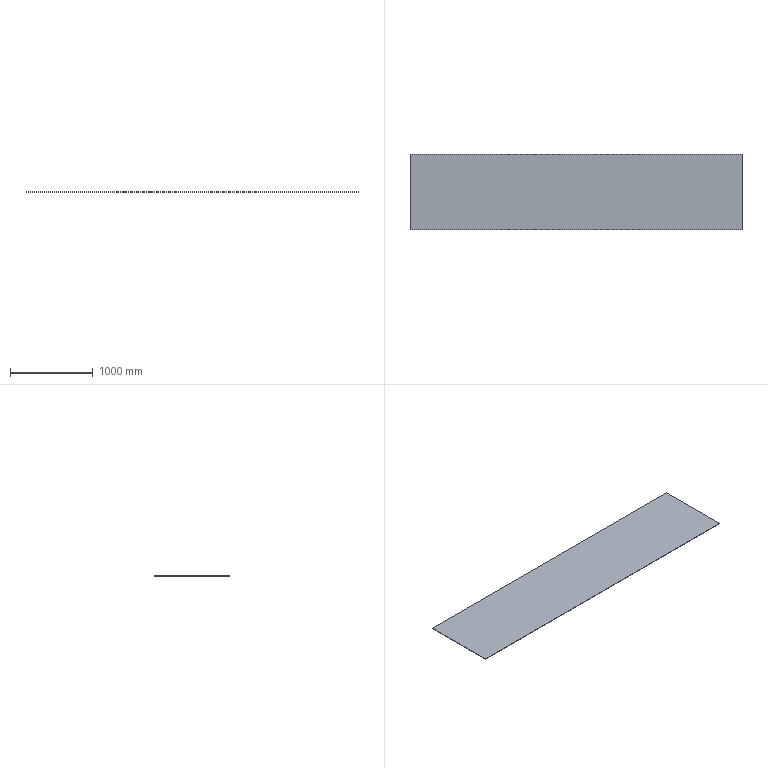Part | SolidWorks | features FlatPattern 1, SMBaseFlange 1, SheetMetal 1 | 1 solid | 6 faces | box 4020 x 910 x 5 mm | volume 18291000 mm3 | plane 6
STEP:
#1=CARTESIAN_POINT('',(0.,910.,0.));
#2=VERTEX_POINT('',#1);
#3=CARTESIAN_POINT('',(0.,0.,0.));
#4=VERTEX_POINT('',#3);
#5=CARTESIAN_POINT('',(0.,0.,0.));
#6=DIRECTION('',(0.,-1.,0.));
#7=VECTOR('',#6,1000.);
#8=LINE('',#5,#7);
#9=EDGE_CURVE('',#2,#4,#8,.T.);
#10=ORIENTED_EDGE('',*,*,#9,.F.);
#11=CARTESIAN_POINT('',(0.,910.,-5.));
#12=VERTEX_POINT('',#11);
#13=CARTESIAN_POINT('',(0.,910.,-5.));
#14=DIRECTION('',(0.,0.,1.));
#15=VECTOR('',#14,1000.);
#16=LINE('',#13,#15);
#17=EDGE_CURVE('',#12,#2,#16,.T.);
#18=ORIENTED_EDGE('',*,*,#17,.F.);
#19=CARTESIAN_POINT('',(0.,0.,-5.));
#20=VERTEX_POINT('',#19);
#21=CARTESIAN_POINT('',(0.,0.,-5.));
#22=DIRECTION('',(0.,-1.,0.));
#23=VECTOR('',#22,1000.);
#24=LINE('',#21,#23);
#25=EDGE_CURVE('',#12,#20,#24,.T.);
#26=ORIENTED_EDGE('',*,*,#25,.T.);
#27=CARTESIAN_POINT('',(0.,0.,-5.));
#28=DIRECTION('',(0.,0.,1.));
#29=VECTOR('',#28,1000.);
#30=LINE('',#27,#29);
#31=EDGE_CURVE('',#20,#4,#30,.T.);
#32=ORIENTED_EDGE('',*,*,#31,.T.);
#33=EDGE_LOOP('',(#10,#18,#26,#32));
#34=FACE_OUTER_BOUND('',#33,.T.);
#35=CARTESIAN_POINT('',(0.,0.,-5.));
#36=DIRECTION('',(-1.,0.,0.));
#37=DIRECTION('',(0.,0.,1.));
#38=AXIS2_PLACEMENT_3D('',#35,#36,#37);
#39=PLANE('',#38);
#40=ADVANCED_FACE('',(#34),#39,.T.);
#41=CARTESIAN_POINT('',(4020.,910.,0.));
#42=VERTEX_POINT('',#41);
#43=CARTESIAN_POINT('',(0.,910.,0.));
#44=DIRECTION('',(-1.,0.,0.));
#45=VECTOR('',#44,1000.);
#46=LINE('',#43,#45);
#47=EDGE_CURVE('',#42,#2,#46,.T.);
#48=ORIENTED_EDGE('',*,*,#47,.F.);
#49=CARTESIAN_POINT('',(4020.,910.,-5.));
#50=VERTEX_POINT('',#49);
#51=CARTESIAN_POINT('',(4020.,910.,-5.));
#52=DIRECTION('',(0.,0.,1.));
#53=VECTOR('',#52,1000.);
#54=LINE('',#51,#53);
#55=EDGE_CURVE('',#50,#42,#54,.T.);
#56=ORIENTED_EDGE('',*,*,#55,.F.);
#57=CARTESIAN_POINT('',(0.,910.,-5.));
#58=DIRECTION('',(-1.,0.,0.));
#59=VECTOR('',#58,1000.);
#60=LINE('',#57,#59);
#61=EDGE_CURVE('',#50,#12,#60,.T.);
#62=ORIENTED_EDGE('',*,*,#61,.T.);
#63=ORIENTED_EDGE('',*,*,#17,.T.);
#64=EDGE_LOOP('',(#48,#56,#62,#63));
#65=FACE_OUTER_BOUND('',#64,.T.);
#66=CARTESIAN_POINT('',(0.,910.,-5.));
#67=DIRECTION('',(0.,1.,0.));
#68=DIRECTION('',(0.,0.,1.));
#69=AXIS2_PLACEMENT_3D('',#66,#67,#68);
#70=PLANE('',#69);
#71=ADVANCED_FACE('',(#65),#70,.T.);
#72=CARTESIAN_POINT('',(4020.,0.,0.));
#73=VERTEX_POINT('',#72);
#74=CARTESIAN_POINT('',(4020.,0.,0.));
#75=DIRECTION('',(0.,1.,0.));
#76=VECTOR('',#75,1000.);
#77=LINE('',#74,#76);
#78=EDGE_CURVE('',#73,#42,#77,.T.);
#79=ORIENTED_EDGE('',*,*,#78,.F.);
#80=CARTESIAN_POINT('',(4020.,0.,-5.));
#81=VERTEX_POINT('',#80);
#82=CARTESIAN_POINT('',(4020.,0.,-5.));
#83=DIRECTION('',(0.,0.,1.));
#84=VECTOR('',#83,1000.);
#85=LINE('',#82,#84);
#86=EDGE_CURVE('',#81,#73,#85,.T.);
#87=ORIENTED_EDGE('',*,*,#86,.F.);
#88=CARTESIAN_POINT('',(4020.,0.,-5.));
#89=DIRECTION('',(0.,1.,0.));
#90=VECTOR('',#89,1000.);
#91=LINE('',#88,#90);
#92=EDGE_CURVE('',#81,#50,#91,.T.);
#93=ORIENTED_EDGE('',*,*,#92,.T.);
#94=ORIENTED_EDGE('',*,*,#55,.T.);
#95=EDGE_LOOP('',(#79,#87,#93,#94));
#96=FACE_OUTER_BOUND('',#95,.T.);
#97=CARTESIAN_POINT('',(4020.,0.,-5.));
#98=DIRECTION('',(1.,0.,0.));
#99=DIRECTION('',(0.,0.,-1.));
#100=AXIS2_PLACEMENT_3D('',#97,#98,#99);
#101=PLANE('',#100);
#102=ADVANCED_FACE('',(#96),#101,.T.);
#103=CARTESIAN_POINT('',(0.,0.,0.));
#104=DIRECTION('',(1.,0.,0.));
#105=VECTOR('',#104,1000.);
#106=LINE('',#103,#105);
#107=EDGE_CURVE('',#4,#73,#106,.T.);
#108=ORIENTED_EDGE('',*,*,#107,.F.);
#109=ORIENTED_EDGE('',*,*,#31,.F.);
#110=CARTESIAN_POINT('',(0.,0.,-5.));
#111=DIRECTION('',(1.,0.,0.));
#112=VECTOR('',#111,1000.);
#113=LINE('',#110,#112);
#114=EDGE_CURVE('',#20,#81,#113,.T.);
#115=ORIENTED_EDGE('',*,*,#114,.T.);
#116=ORIENTED_EDGE('',*,*,#86,.T.);
#117=EDGE_LOOP('',(#108,#109,#115,#116));
#118=FACE_OUTER_BOUND('',#117,.T.);
#119=CARTESIAN_POINT('',(0.,0.,-5.));
#120=DIRECTION('',(0.,-1.,0.));
#121=DIRECTION('',(0.,0.,-1.));
#122=AXIS2_PLACEMENT_3D('',#119,#120,#121);
#123=PLANE('',#122);
#124=ADVANCED_FACE('',(#118),#123,.T.);
#125=ORIENTED_EDGE('',*,*,#25,.F.);
#126=ORIENTED_EDGE('',*,*,#61,.F.);
#127=ORIENTED_EDGE('',*,*,#92,.F.);
#128=ORIENTED_EDGE('',*,*,#114,.F.);
#129=EDGE_LOOP('',(#125,#126,#127,#128));
#130=FACE_OUTER_BOUND('',#129,.T.);
#131=CARTESIAN_POINT('',(0.,0.,-5.));
#132=DIRECTION('',(0.,0.,-1.));
#133=DIRECTION('',(-1.,0.,0.));
#134=AXIS2_PLACEMENT_3D('',#131,#132,#133);
#135=PLANE('',#134);
#136=ADVANCED_FACE('',(#130),#135,.T.);
#137=ORIENTED_EDGE('',*,*,#9,.T.);
#138=ORIENTED_EDGE('',*,*,#107,.T.);
#139=ORIENTED_EDGE('',*,*,#78,.T.);
#140=ORIENTED_EDGE('',*,*,#47,.T.);
#141=EDGE_LOOP('',(#137,#138,#139,#140));
#142=FACE_OUTER_BOUND('',#141,.T.);
#143=CARTESIAN_POINT('',(0.,0.,0.));
#144=DIRECTION('',(0.,0.,-1.));
#145=DIRECTION('',(-1.,0.,0.));
#146=AXIS2_PLACEMENT_3D('',#143,#144,#145);
#147=PLANE('',#146);
#148=ADVANCED_FACE('',(#142),#147,.F.);
#149=CLOSED_SHELL('',(#40,#71,#102,#124,#136,#148));
#150=MANIFOLD_SOLID_BREP('',#149);
#151=CARTESIAN_POINT('',(0.,0.,0.));
#152=DIRECTION('',(0.,0.,1.));
#153=DIRECTION('',(1.,0.,0.));
#154=AXIS2_PLACEMENT_3D('',#151,#152,#153);
#155=(LENGTH_UNIT()NAMED_UNIT(*)SI_UNIT(.MILLI.,.METRE.));
#156=UNCERTAINTY_MEASURE_WITH_UNIT(LENGTH_MEASURE(0.00001),#155,'','');
#157=(NAMED_UNIT(*)PLANE_ANGLE_UNIT()SI_UNIT($,.RADIAN.));
#158=(NAMED_UNIT(*)SI_UNIT($,.STERADIAN.)SOLID_ANGLE_UNIT());
#159=(GEOMETRIC_REPRESENTATION_CONTEXT(3)GLOBAL_UNCERTAINTY_ASSIGNED_CONTEXT((#156))GLOBAL_UNIT_ASSIGNED_CONTEXT((#155,#157,#158))REPRESENTATION_CONTEXT('',''));
#160=ADVANCED_BREP_SHAPE_REPRESENTATION('',(#150,#154),#159);